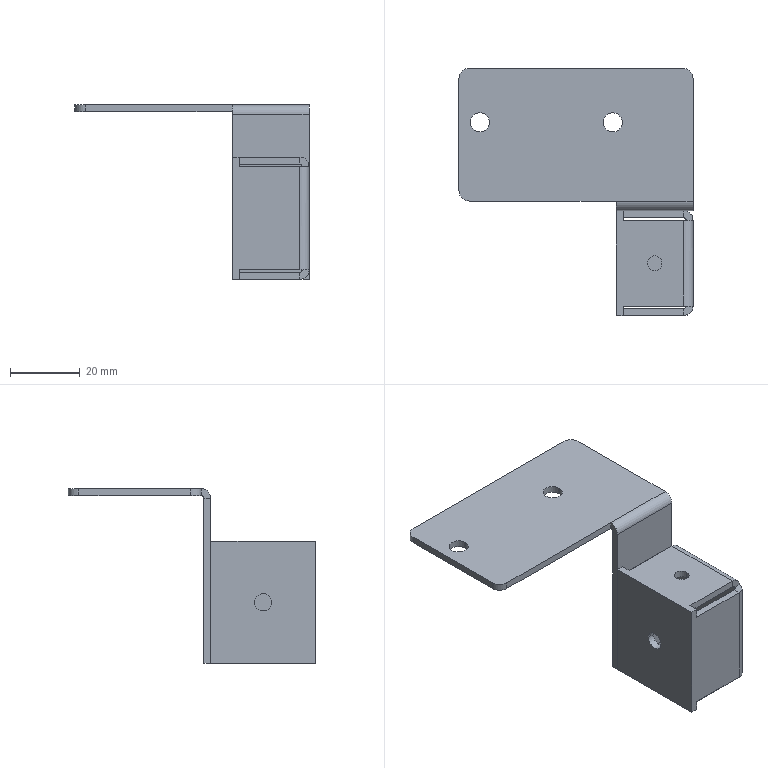Part | SolidWorks | features ICE 4, EdgeFlange 2, FlatPattern 2, HoleWzd 2, SMBaseFlange 2, SheetMetal 2, Fillet 1 | 2 solids | 66 faces | box 67 x 70.75 x 50 mm | volume 14918 mm3 | plane 33 | cylinder 25 | spline 8 | commonest cylinder face diameters 5.5 x9 5 x6 1.5 x5 6 x3 4.2 x2